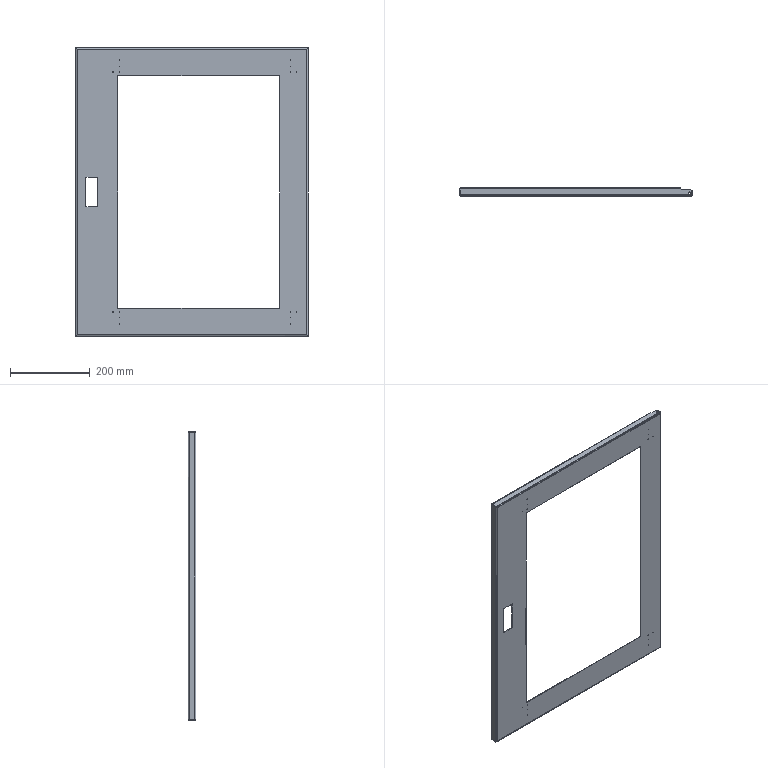Part | NX | features solid 2 | 1 solid | 142 faces | box 581 x 20 x 721 mm | volume 366405 mm3 | plane 68 | cylinder 50 | spline 24 | commonest cylinder face diameters 1 x32 6 x11 3 x7